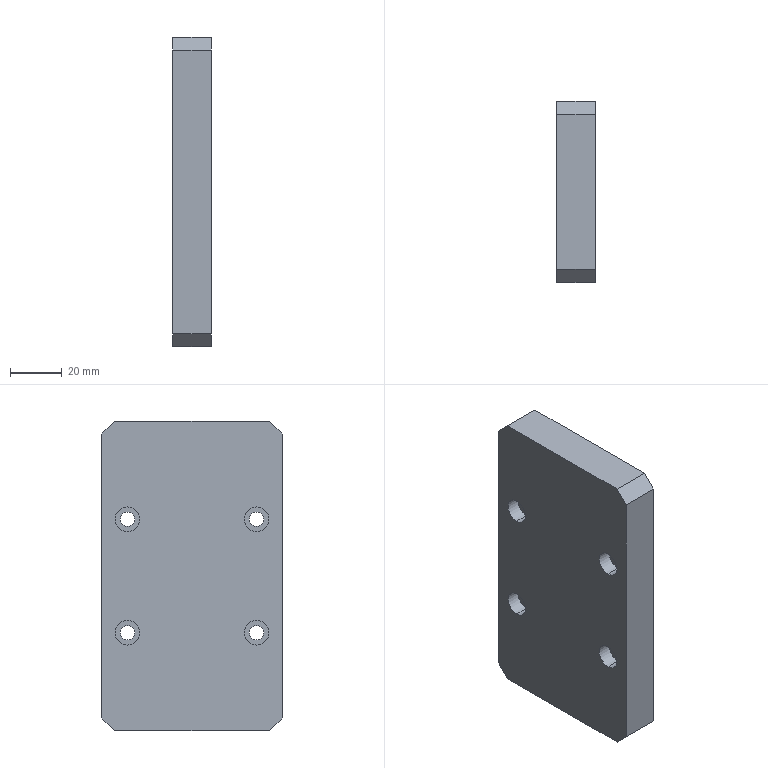Part | STEP file | CLAMP.ARM.3.stp | 1 solid | 30 faces | box 15 x 70 x 120 mm | volume 122807 mm3 | plane 12 | spline 10 | cylinder 8 | commonest cylinder face diameters 5.5 x4 9.5 x4